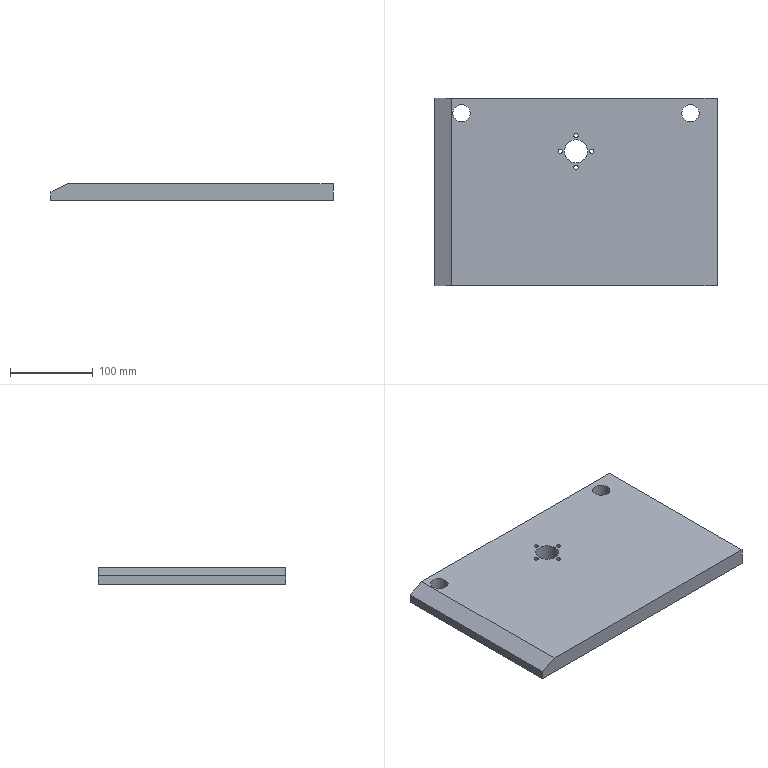Part | STEP file | 0230_202_Guide | 1 solid | 29 faces | box 340 x 226 x 20.4 mm | volume 1516540 mm3 | cylinder 18 | plane 7 | cone 4 | commonest cylinder face diameters 5 x8 2.5 x4 21 x4 28 x2